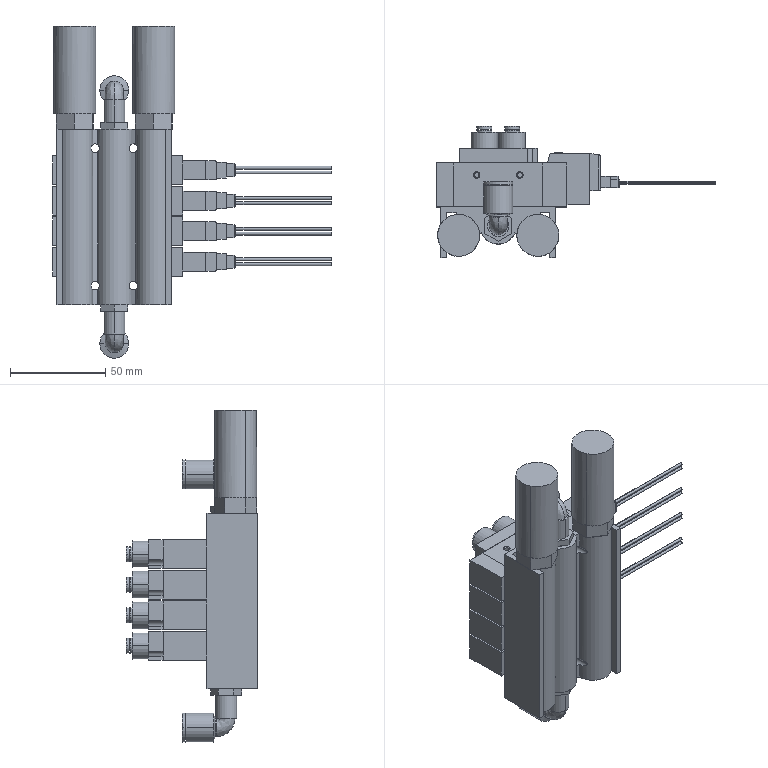Part | SolidWorks | features ReferencePattern 3, AEMSimFeature 1, LocalLPattern 1 | 11 solids | 885 faces | box 146.05 x 68.7 x 173.94 mm | volume 268514 mm3 | plane 491 | cylinder 270 | cone 120 | spline 4 | commonest cylinder face diameters 7.9 x32 6.2 x24 8.57 x24 1.5 x16 2.46 x16 2.5 x16